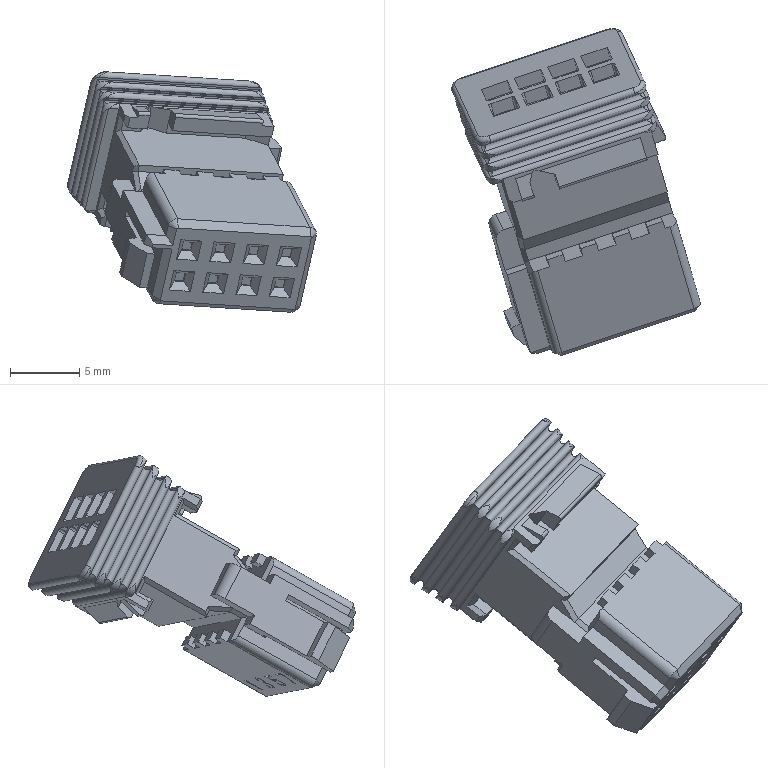Part | SolidWorks | features BaseBody 1 | 1 solid | 457 faces | box 17.995 x 23.635 x 17.388 mm | volume 1594 mm3 | plane 365 | cylinder 72 | spline 12 | cone 4 | torus 4 | commonest cylinder face diameters 0.6 x26 0.4 x21 0.602 x8 0.617 x4 0.618 x4 1.2 x4